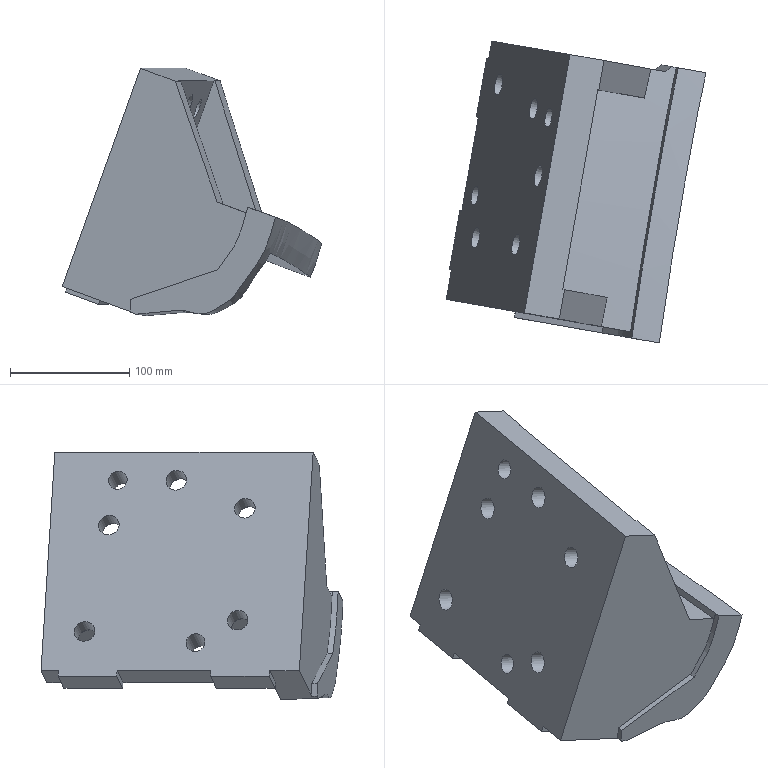Part | NX | features solid 2 | 1 solid | 53 faces | box 217.946 x 253.516 x 207.673 mm | volume 2484321 mm3 | plane 33 | cylinder 12 | spline 8 | commonest cylinder face diameters 17.5 x5 25 x5 16 x2